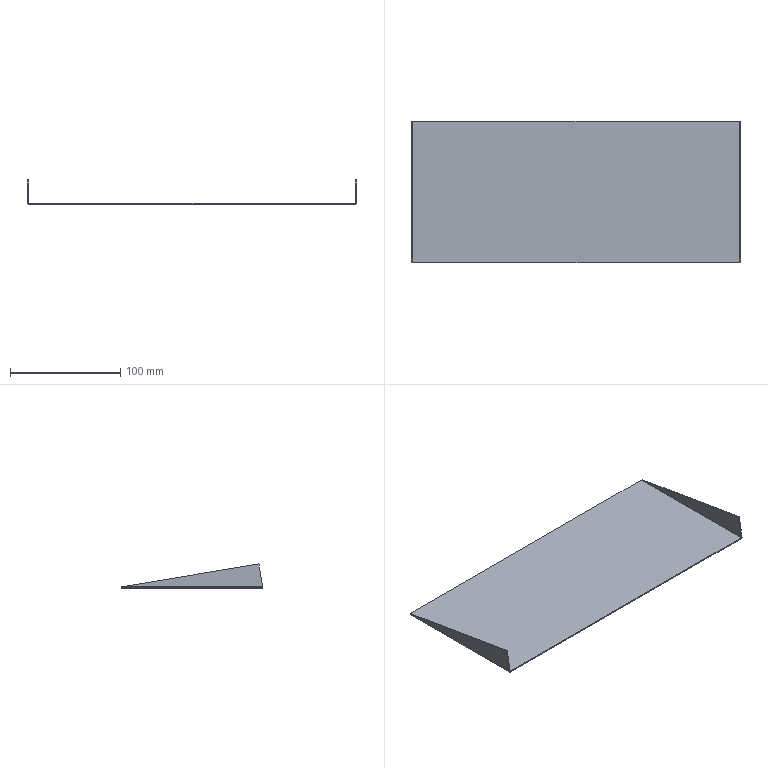Part | SolidWorks | features EdgeFlange 1, FlatPattern 1, MirrorPattern 1, SMBaseFlange 1, SheetMetal 1 | 1 solid | 20 faces | box 299 x 128.5 x 22 mm | volume 41042 mm3 | plane 12 | spline 4 | cylinder 4 | commonest cylinder face diameters 0.4 x2 2.4 x2
STEP:
#1=CARTESIAN_POINT('',(148.3,64.25,-1.));
#2=VERTEX_POINT('',#1);
#3=CARTESIAN_POINT('',(148.3,-64.25,-1.));
#4=VERTEX_POINT('',#3);
#5=CARTESIAN_POINT('',(148.3,64.25,-1.));
#6=DIRECTION('',(0.,-1.,0.));
#7=VECTOR('',#6,1000.);
#8=LINE('',#5,#7);
#9=EDGE_CURVE('',#2,#4,#8,.T.);
#10=ORIENTED_EDGE('',*,*,#9,.T.);
#11=CARTESIAN_POINT('',(-148.3,-64.25,-1.));
#12=VERTEX_POINT('',#11);
#13=CARTESIAN_POINT('',(-149.5,-64.25,-1.));
#14=DIRECTION('',(1.,0.,0.));
#15=VECTOR('',#14,1000.);
#16=LINE('',#13,#15);
#17=EDGE_CURVE('',#12,#4,#16,.T.);
#18=ORIENTED_EDGE('',*,*,#17,.F.);
#19=CARTESIAN_POINT('',(-148.3,64.25,-1.));
#20=VERTEX_POINT('',#19);
#21=CARTESIAN_POINT('',(-148.3,-64.25,-1.));
#22=DIRECTION('',(0.,1.,0.));
#23=VECTOR('',#22,1000.);
#24=LINE('',#21,#23);
#25=EDGE_CURVE('',#12,#20,#24,.T.);
#26=ORIENTED_EDGE('',*,*,#25,.T.);
#27=CARTESIAN_POINT('',(-149.5,64.25,-1.));
#28=DIRECTION('',(-1.,0.,0.));
#29=VECTOR('',#28,1000.);
#30=LINE('',#27,#29);
#31=EDGE_CURVE('',#2,#20,#30,.T.);
#32=ORIENTED_EDGE('',*,*,#31,.F.);
#33=EDGE_LOOP('',(#10,#18,#26,#32));
#34=FACE_OUTER_BOUND('',#33,.T.);
#35=CARTESIAN_POINT('',(0.,0.,-1.));
#36=DIRECTION('',(0.,0.,1.));
#37=DIRECTION('',(1.,0.,0.));
#38=AXIS2_PLACEMENT_3D('',#35,#36,#37);
#39=PLANE('',#38);
#40=ADVANCED_FACE('',(#34),#39,.F.);
#41=CARTESIAN_POINT('',(-148.3,-64.25,0.));
#42=VERTEX_POINT('',#41);
#43=CARTESIAN_POINT('',(148.3,-64.25,0.));
#44=VERTEX_POINT('',#43);
#45=CARTESIAN_POINT('',(-149.5,-64.25,0.));
#46=DIRECTION('',(1.,0.,0.));
#47=VECTOR('',#46,1000.);
#48=LINE('',#45,#47);
#49=EDGE_CURVE('',#42,#44,#48,.T.);
#50=ORIENTED_EDGE('',*,*,#49,.T.);
#51=CARTESIAN_POINT('',(148.3,64.25,0.));
#52=VERTEX_POINT('',#51);
#53=CARTESIAN_POINT('',(148.3,64.25,0.));
#54=DIRECTION('',(0.,-1.,0.));
#55=VECTOR('',#54,1000.);
#56=LINE('',#53,#55);
#57=EDGE_CURVE('',#52,#44,#56,.T.);
#58=ORIENTED_EDGE('',*,*,#57,.F.);
#59=CARTESIAN_POINT('',(-148.3,64.25,0.));
#60=VERTEX_POINT('',#59);
#61=CARTESIAN_POINT('',(-149.5,64.25,0.));
#62=DIRECTION('',(-1.,0.,0.));
#63=VECTOR('',#62,1000.);
#64=LINE('',#61,#63);
#65=EDGE_CURVE('',#52,#60,#64,.T.);
#66=ORIENTED_EDGE('',*,*,#65,.T.);
#67=CARTESIAN_POINT('',(-148.3,-64.25,0.));
#68=DIRECTION('',(0.,1.,0.));
#69=VECTOR('',#68,1000.);
#70=LINE('',#67,#69);
#71=EDGE_CURVE('',#42,#60,#70,.T.);
#72=ORIENTED_EDGE('',*,*,#71,.F.);
#73=EDGE_LOOP('',(#50,#58,#66,#72));
#74=FACE_OUTER_BOUND('',#73,.T.);
#75=CARTESIAN_POINT('',(0.,0.,0.));
#76=DIRECTION('',(0.,0.,1.));
#77=DIRECTION('',(1.,0.,0.));
#78=AXIS2_PLACEMENT_3D('',#75,#76,#77);
#79=PLANE('',#78);
#80=ADVANCED_FACE('',(#74),#79,.T.);
#81=ORIENTED_EDGE('',*,*,#65,.F.);
#82=CARTESIAN_POINT('',(148.3,64.25,0.));
#83=DIRECTION('',(0.,0.,-1.));
#84=VECTOR('',#83,1000.);
#85=LINE('',#82,#84);
#86=EDGE_CURVE('',#52,#2,#85,.T.);
#87=ORIENTED_EDGE('',*,*,#86,.T.);
#88=ORIENTED_EDGE('',*,*,#31,.T.);
#89=CARTESIAN_POINT('',(-148.3,64.25,0.));
#90=DIRECTION('',(0.,0.,-1.));
#91=VECTOR('',#90,1000.);
#92=LINE('',#89,#91);
#93=EDGE_CURVE('',#60,#20,#92,.T.);
#94=ORIENTED_EDGE('',*,*,#93,.F.);
#95=EDGE_LOOP('',(#81,#87,#88,#94));
#96=FACE_OUTER_BOUND('',#95,.T.);
#97=CARTESIAN_POINT('',(-149.5,64.25,-1.));
#98=DIRECTION('',(0.,1.,0.));
#99=DIRECTION('',(0.,0.,1.));
#100=AXIS2_PLACEMENT_3D('',#97,#98,#99);
#101=PLANE('',#100);
#102=ADVANCED_FACE('',(#96),#101,.T.);
#103=CARTESIAN_POINT('',(148.3,-64.25,0.));
#104=DIRECTION('',(0.,0.,-1.));
#105=VECTOR('',#104,1000.);
#106=LINE('',#103,#105);
#107=EDGE_CURVE('',#44,#4,#106,.T.);
#108=ORIENTED_EDGE('',*,*,#107,.F.);
#109=ORIENTED_EDGE('',*,*,#49,.F.);
#110=CARTESIAN_POINT('',(-148.3,-64.25,0.));
#111=DIRECTION('',(0.,0.,-1.));
#112=VECTOR('',#111,1000.);
#113=LINE('',#110,#112);
#114=EDGE_CURVE('',#42,#12,#113,.T.);
#115=ORIENTED_EDGE('',*,*,#114,.T.);
#116=ORIENTED_EDGE('',*,*,#17,.T.);
#117=EDGE_LOOP('',(#108,#109,#115,#116));
#118=FACE_OUTER_BOUND('',#117,.T.);
#119=CARTESIAN_POINT('',(-149.5,-64.25,-1.));
#120=DIRECTION('',(0.,-1.,0.));
#121=DIRECTION('',(0.,0.,-1.));
#122=AXIS2_PLACEMENT_3D('',#119,#120,#121);
#123=PLANE('',#122);
#124=ADVANCED_FACE('',(#118),#123,.T.);
#125=CARTESIAN_POINT('',(-148.5,63.06,0.2));
#126=VERTEX_POINT('',#125);
#127=CARTESIAN_POINT('',(-149.5,63.06,0.2));
#128=VERTEX_POINT('',#127);
#129=CARTESIAN_POINT('',(-149.5,63.06,0.2));
#130=DIRECTION('',(-1.,0.,0.));
#131=VECTOR('',#130,1000.);
#132=LINE('',#129,#131);
#133=EDGE_CURVE('',#126,#128,#132,.T.);
#134=ORIENTED_EDGE('',*,*,#133,.F.);
#135=CARTESIAN_POINT('',(-148.3,64.25,0.));
#136=CARTESIAN_POINT('',(-148.352,64.052,0.));
#137=CARTESIAN_POINT('',(-148.404,63.853,0.02155));
#138=CARTESIAN_POINT('',(-148.478,63.457,0.0956));
#139=CARTESIAN_POINT('',(-148.5,63.258,0.1476));
#140=CARTESIAN_POINT('',(-148.5,63.06,0.2));
#141=B_SPLINE_CURVE_WITH_KNOTS('',3,(#135,#136,#137,#138,#139,#140),.UNSPECIFIED.,.F.,.F.,(4,2,4),(0.,0.5,1.),.UNSPECIFIED.);
#142=EDGE_CURVE('',#60,#126,#141,.T.);
#143=ORIENTED_EDGE('',*,*,#142,.F.);
#144=ORIENTED_EDGE('',*,*,#93,.T.);
#145=CARTESIAN_POINT('',(-148.3,64.25,-1.));
#146=CARTESIAN_POINT('',(-148.459,64.15,-1.));
#147=CARTESIAN_POINT('',(-148.614,64.052,-0.9688));
#148=CARTESIAN_POINT('',(-148.906,63.852,-0.8478));
#149=CARTESIAN_POINT('',(-149.037,63.754,-0.7598));
#150=CARTESIAN_POINT('',(-149.261,63.555,-0.5362));
#151=CARTESIAN_POINT('',(-149.348,63.457,-0.4048));
#152=CARTESIAN_POINT('',(-149.469,63.257,-0.1126));
#153=CARTESIAN_POINT('',(-149.5,63.16,0.04146));
#154=CARTESIAN_POINT('',(-149.5,63.06,0.2));
#155=B_SPLINE_CURVE_WITH_KNOTS('',3,(#145,#146,#147,#148,#149,#150,#151,#152,#153,#154),.UNSPECIFIED.,.F.,.F.,(4,2,2,2,4),(0.,0.000556,0.001112,0.001668,0.002224),.UNSPECIFIED.);
#156=EDGE_CURVE('',#20,#128,#155,.T.);
#157=ORIENTED_EDGE('',*,*,#156,.T.);
#158=EDGE_LOOP('',(#134,#143,#144,#157));
#159=FACE_OUTER_BOUND('',#158,.T.);
#160=CARTESIAN_POINT('',(-148.3,64.25,-1.01));
#161=CARTESIAN_POINT('',(-148.458,64.151,-1.01));
#162=CARTESIAN_POINT('',(-148.617,64.052,-0.9785));
#163=CARTESIAN_POINT('',(-148.909,63.853,-0.8573));
#164=CARTESIAN_POINT('',(-149.044,63.754,-0.7676));
#165=CARTESIAN_POINT('',(-149.268,63.556,-0.5436));
#166=CARTESIAN_POINT('',(-149.357,63.457,-0.4094));
#167=CARTESIAN_POINT('',(-149.479,63.258,-0.1167));
#168=CARTESIAN_POINT('',(-149.51,63.159,0.04159));
#169=CARTESIAN_POINT('',(-149.51,63.06,0.2));
#170=CARTESIAN_POINT('',(-148.3,64.25,-1.));
#171=CARTESIAN_POINT('',(-148.457,64.151,-1.));
#172=CARTESIAN_POINT('',(-148.614,64.052,-0.9688));
#173=CARTESIAN_POINT('',(-148.904,63.853,-0.8485));
#174=CARTESIAN_POINT('',(-149.037,63.754,-0.7596));
#175=CARTESIAN_POINT('',(-149.26,63.556,-0.5375));
#176=CARTESIAN_POINT('',(-149.349,63.457,-0.4043));
#177=CARTESIAN_POINT('',(-149.469,63.258,-0.1141));
#178=CARTESIAN_POINT('',(-149.5,63.159,0.0429));
#179=CARTESIAN_POINT('',(-149.5,63.06,0.2));
#180=CARTESIAN_POINT('',(-148.3,64.25,0.));
#181=CARTESIAN_POINT('',(-148.326,64.151,0.));
#182=CARTESIAN_POINT('',(-148.352,64.052,0.005205));
#183=CARTESIAN_POINT('',(-148.401,63.853,0.02524));
#184=CARTESIAN_POINT('',(-148.423,63.754,0.04007));
#185=CARTESIAN_POINT('',(-148.46,63.556,0.07709));
#186=CARTESIAN_POINT('',(-148.475,63.457,0.09928));
#187=CARTESIAN_POINT('',(-148.495,63.258,0.1477));
#188=CARTESIAN_POINT('',(-148.5,63.159,0.1738));
#189=CARTESIAN_POINT('',(-148.5,63.06,0.2));
#190=B_SPLINE_SURFACE_WITH_KNOTS('',1,3,((#160,#161,#162,#163,#164,#165,#166,#167,#168,#169),(#170,#171,#172,#173,#174,#175,#176,#177,#178,#179),(#180,#181,#182,#183,#184,#185,#186,#187,#188,#189)),.UNSPECIFIED.,.F.,.F.,.F.,(2,1,2),(4,2,2,2,4),(-0.01,0.,1.),(0.,0.25,0.5,0.75,1.),.UNSPECIFIED.);
#191=ADVANCED_FACE('',(#159),#190,.F.);
#192=CARTESIAN_POINT('',(-148.5,-64.216,0.2));
#193=VERTEX_POINT('',#192);
#194=CARTESIAN_POINT('',(-148.5,-64.216,0.2));
#195=CARTESIAN_POINT('',(-148.5,-64.222,0.1476));
#196=CARTESIAN_POINT('',(-148.478,-64.228,0.0956));
#197=CARTESIAN_POINT('',(-148.404,-64.239,0.02155));
#198=CARTESIAN_POINT('',(-148.352,-64.244,0.));
#199=CARTESIAN_POINT('',(-148.3,-64.25,0.));
#200=B_SPLINE_CURVE_WITH_KNOTS('',3,(#194,#195,#196,#197,#198,#199),.UNSPECIFIED.,.F.,.F.,(4,2,4),(0.,0.5,1.),.UNSPECIFIED.);
#201=EDGE_CURVE('',#193,#42,#200,.T.);
#202=ORIENTED_EDGE('',*,*,#201,.F.);
#203=CARTESIAN_POINT('',(-149.5,-64.216,0.2));
#204=VERTEX_POINT('',#203);
#205=CARTESIAN_POINT('',(-148.5,-64.216,0.2));
#206=DIRECTION('',(-1.,0.,0.));
#207=VECTOR('',#206,1000.);
#208=LINE('',#205,#207);
#209=EDGE_CURVE('',#193,#204,#208,.T.);
#210=ORIENTED_EDGE('',*,*,#209,.T.);
#211=CARTESIAN_POINT('',(-149.5,-64.216,0.2));
#212=CARTESIAN_POINT('',(-149.5,-64.219,0.04292));
#213=CARTESIAN_POINT('',(-149.469,-64.222,-0.1141));
#214=CARTESIAN_POINT('',(-149.349,-64.228,-0.4043));
#215=CARTESIAN_POINT('',(-149.26,-64.23,-0.5375));
#216=CARTESIAN_POINT('',(-149.037,-64.236,-0.7596));
#217=CARTESIAN_POINT('',(-148.904,-64.239,-0.8485));
#218=CARTESIAN_POINT('',(-148.614,-64.244,-0.9688));
#219=CARTESIAN_POINT('',(-148.457,-64.247,-1.));
#220=CARTESIAN_POINT('',(-148.3,-64.25,-1.));
#221=B_SPLINE_CURVE_WITH_KNOTS('',3,(#211,#212,#213,#214,#215,#216,#217,#218,#219,#220),.UNSPECIFIED.,.F.,.F.,(4,2,2,2,4),(0.,0.25,0.5,0.75,1.),.UNSPECIFIED.);
#222=EDGE_CURVE('',#204,#12,#221,.T.);
#223=ORIENTED_EDGE('',*,*,#222,.T.);
#224=ORIENTED_EDGE('',*,*,#114,.F.);
#225=EDGE_LOOP('',(#202,#210,#223,#224));
#226=FACE_OUTER_BOUND('',#225,.T.);
#227=CARTESIAN_POINT('',(-149.51,-64.216,0.2));
#228=CARTESIAN_POINT('',(-149.51,-64.219,0.04158));
#229=CARTESIAN_POINT('',(-149.479,-64.222,-0.1167));
#230=CARTESIAN_POINT('',(-149.357,-64.228,-0.4094));
#231=CARTESIAN_POINT('',(-149.268,-64.23,-0.5436));
#232=CARTESIAN_POINT('',(-149.044,-64.236,-0.7676));
#233=CARTESIAN_POINT('',(-148.909,-64.239,-0.8573));
#234=CARTESIAN_POINT('',(-148.617,-64.244,-0.9785));
#235=CARTESIAN_POINT('',(-148.458,-64.247,-1.01));
#236=CARTESIAN_POINT('',(-148.3,-64.25,-1.01));
#237=CARTESIAN_POINT('',(-149.5,-64.216,0.2));
#238=CARTESIAN_POINT('',(-149.5,-64.219,0.04289));
#239=CARTESIAN_POINT('',(-149.469,-64.222,-0.1141));
#240=CARTESIAN_POINT('',(-149.349,-64.228,-0.4043));
#241=CARTESIAN_POINT('',(-149.26,-64.23,-0.5375));
#242=CARTESIAN_POINT('',(-149.037,-64.236,-0.7596));
#243=CARTESIAN_POINT('',(-148.904,-64.239,-0.8485));
#244=CARTESIAN_POINT('',(-148.614,-64.244,-0.9688));
#245=CARTESIAN_POINT('',(-148.457,-64.247,-1.));
#246=CARTESIAN_POINT('',(-148.3,-64.25,-1.));
#247=CARTESIAN_POINT('',(-148.5,-64.216,0.2));
#248=CARTESIAN_POINT('',(-148.5,-64.219,0.1738));
#249=CARTESIAN_POINT('',(-148.495,-64.222,0.1477));
#250=CARTESIAN_POINT('',(-148.475,-64.228,0.09928));
#251=CARTESIAN_POINT('',(-148.46,-64.23,0.07709));
#252=CARTESIAN_POINT('',(-148.423,-64.236,0.04007));
#253=CARTESIAN_POINT('',(-148.401,-64.239,0.02524));
#254=CARTESIAN_POINT('',(-148.352,-64.244,0.005205));
#255=CARTESIAN_POINT('',(-148.326,-64.247,0.));
#256=CARTESIAN_POINT('',(-148.3,-64.25,0.));
#257=CARTESIAN_POINT('',(-148.49,-64.216,0.2));
#258=CARTESIAN_POINT('',(-148.49,-64.219,0.1751));
#259=CARTESIAN_POINT('',(-148.485,-64.222,0.1503));
#260=CARTESIAN_POINT('',(-148.466,-64.228,0.1044));
#261=CARTESIAN_POINT('',(-148.452,-64.23,0.0833));
#262=CARTESIAN_POINT('',(-148.417,-64.236,0.04814));
#263=CARTESIAN_POINT('',(-148.396,-64.239,0.03407));
#264=CARTESIAN_POINT('',(-148.35,-64.244,0.01504));
#265=CARTESIAN_POINT('',(-148.325,-64.247,0.0101));
#266=CARTESIAN_POINT('',(-148.3,-64.25,0.0101));
#267=B_SPLINE_SURFACE_WITH_KNOTS('',1,3,((#227,#228,#229,#230,#231,#232,#233,#234,#235,#236),(#237,#238,#239,#240,#241,#242,#243,#244,#245,#246),(#247,#248,#249,#250,#251,#252,#253,#254,#255,#256),(#257,#258,#259,#260,#261,#262,#263,#264,#265,#266)),.UNSPECIFIED.,.F.,.F.,.F.,(2,1,1,2),(4,2,2,2,4),(-0.01,0.,1.,1.01),(0.,0.25,0.5,0.75,1.),.UNSPECIFIED.);
#268=ADVANCED_FACE('',(#226),#267,.F.);
#269=ORIENTED_EDGE('',*,*,#25,.F.);
#270=ORIENTED_EDGE('',*,*,#222,.F.);
#271=CARTESIAN_POINT('',(-149.5,63.06,0.2));
#272=DIRECTION('',(0.,1.,0.));
#273=VECTOR('',#272,1000.);
#274=LINE('',#271,#273);
#275=EDGE_CURVE('',#204,#128,#274,.T.);
#276=ORIENTED_EDGE('',*,*,#275,.T.);
#277=ORIENTED_EDGE('',*,*,#156,.F.);
#278=EDGE_LOOP('',(#269,#270,#276,#277));
#279=FACE_OUTER_BOUND('',#278,.T.);
#280=CARTESIAN_POINT('',(-148.3,-64.25,0.2));
#281=DIRECTION('',(0.,-1.,0.));
#282=DIRECTION('',(-1.,0.,0.));
#283=AXIS2_PLACEMENT_3D('',#280,#281,#282);
#284=CYLINDRICAL_SURFACE('',#283,1.2);
#285=ADVANCED_FACE('',(#279),#284,.T.);
#286=ORIENTED_EDGE('',*,*,#71,.T.);
#287=ORIENTED_EDGE('',*,*,#142,.T.);
#288=CARTESIAN_POINT('',(-148.5,63.06,0.2));
#289=DIRECTION('',(0.,-1.,0.));
#290=VECTOR('',#289,1000.);
#291=LINE('',#288,#290);
#292=EDGE_CURVE('',#126,#193,#291,.T.);
#293=ORIENTED_EDGE('',*,*,#292,.T.);
#294=ORIENTED_EDGE('',*,*,#201,.T.);
#295=EDGE_LOOP('',(#286,#287,#293,#294));
#296=FACE_OUTER_BOUND('',#295,.T.);
#297=CARTESIAN_POINT('',(-148.3,-64.25,0.2));
#298=DIRECTION('',(0.,-1.,0.));
#299=DIRECTION('',(-1.,0.,0.));
#300=AXIS2_PLACEMENT_3D('',#297,#298,#299);
#301=CYLINDRICAL_SURFACE('',#300,0.2);
#302=ADVANCED_FACE('',(#296),#301,.F.);
#303=ORIENTED_EDGE('',*,*,#133,.T.);
#304=CARTESIAN_POINT('',(-149.5,-60.721,21.));
#305=VERTEX_POINT('',#304);
#306=CARTESIAN_POINT('',(-149.5,1.764,10.5));
#307=DIRECTION('',(0.,0.9862,-0.1657));
#308=VECTOR('',#307,1000.);
#309=LINE('',#306,#308);
#310=EDGE_CURVE('',#305,#128,#309,.T.);
#311=ORIENTED_EDGE('',*,*,#310,.F.);
#312=CARTESIAN_POINT('',(-148.5,-60.721,21.));
#313=VERTEX_POINT('',#312);
#314=CARTESIAN_POINT('',(-149.5,-60.721,21.));
#315=DIRECTION('',(1.,0.,0.));
#316=VECTOR('',#315,1000.);
#317=LINE('',#314,#316);
#318=EDGE_CURVE('',#305,#313,#317,.T.);
#319=ORIENTED_EDGE('',*,*,#318,.T.);
#320=CARTESIAN_POINT('',(-148.5,-60.721,21.));
#321=DIRECTION('',(0.,0.9862,-0.1657));
#322=VECTOR('',#321,1000.);
#323=LINE('',#320,#322);
#324=EDGE_CURVE('',#313,#126,#323,.T.);
#325=ORIENTED_EDGE('',*,*,#324,.T.);
#326=EDGE_LOOP('',(#303,#311,#319,#325));
#327=FACE_OUTER_BOUND('',#326,.T.);
#328=CARTESIAN_POINT('',(-149.5,-60.721,21.));
#329=DIRECTION('',(0.,-0.1657,-0.9862));
#330=DIRECTION('',(0.,0.9862,-0.1657));
#331=AXIS2_PLACEMENT_3D('',#328,#329,#330);
#332=PLANE('',#331);
#333=ADVANCED_FACE('',(#327),#332,.F.);
#334=ORIENTED_EDGE('',*,*,#209,.F.);
#335=CARTESIAN_POINT('',(-148.5,-64.25,0.));
#336=DIRECTION('',(0.,0.1657,0.9862));
#337=VECTOR('',#336,1000.);
#338=LINE('',#335,#337);
#339=EDGE_CURVE('',#193,#313,#338,.T.);
#340=ORIENTED_EDGE('',*,*,#339,.T.);
#341=ORIENTED_EDGE('',*,*,#318,.F.);
#342=CARTESIAN_POINT('',(-149.5,-62.486,10.5));
#343=DIRECTION('',(0.,0.1657,0.9862));
#344=VECTOR('',#343,1000.);
#345=LINE('',#342,#344);
#346=EDGE_CURVE('',#204,#305,#345,.T.);
#347=ORIENTED_EDGE('',*,*,#346,.F.);
#348=EDGE_LOOP('',(#334,#340,#341,#347));
#349=FACE_OUTER_BOUND('',#348,.T.);
#350=CARTESIAN_POINT('',(-149.5,-64.25,0.));
#351=DIRECTION('',(0.,0.9862,-0.1657));
#352=DIRECTION('',(0.,0.1657,0.9862));
#353=AXIS2_PLACEMENT_3D('',#350,#351,#352);
#354=PLANE('',#353);
#355=ADVANCED_FACE('',(#349),#354,.F.);
#356=ORIENTED_EDGE('',*,*,#275,.F.);
#357=ORIENTED_EDGE('',*,*,#346,.T.);
#358=ORIENTED_EDGE('',*,*,#310,.T.);
#359=EDGE_LOOP('',(#356,#357,#358));
#360=FACE_OUTER_BOUND('',#359,.T.);
#361=CARTESIAN_POINT('',(-149.5,0.,0.));
#362=DIRECTION('',(1.,0.,0.));
#363=DIRECTION('',(0.,0.,-1.));
#364=AXIS2_PLACEMENT_3D('',#361,#362,#363);
#365=PLANE('',#364);
#366=ADVANCED_FACE('',(#360),#365,.F.);
#367=ORIENTED_EDGE('',*,*,#339,.F.);
#368=ORIENTED_EDGE('',*,*,#292,.F.);
#369=ORIENTED_EDGE('',*,*,#324,.F.);
#370=EDGE_LOOP('',(#367,#368,#369));
#371=FACE_OUTER_BOUND('',#370,.T.);
#372=CARTESIAN_POINT('',(-148.5,0.,0.));
#373=DIRECTION('',(1.,0.,0.));
#374=DIRECTION('',(0.,0.,-1.));
#375=AXIS2_PLACEMENT_3D('',#372,#373,#374);
#376=PLANE('',#375);
#377=ADVANCED_FACE('',(#371),#376,.T.);
#378=CARTESIAN_POINT('',(148.5,-64.216,0.2));
#379=VERTEX_POINT('',#378);
#380=CARTESIAN_POINT('',(149.5,-64.216,0.2));
#381=VERTEX_POINT('',#380);
#382=CARTESIAN_POINT('',(149.5,-64.216,0.2));
#383=DIRECTION('',(1.,0.,0.));
#384=VECTOR('',#383,1000.);
#385=LINE('',#382,#384);
#386=EDGE_CURVE('',#379,#381,#385,.T.);
#387=ORIENTED_EDGE('',*,*,#386,.F.);
#388=CARTESIAN_POINT('',(148.3,-64.25,0.));
#389=CARTESIAN_POINT('',(148.352,-64.244,0.));
#390=CARTESIAN_POINT('',(148.404,-64.239,0.02155));
#391=CARTESIAN_POINT('',(148.478,-64.228,0.0956));
#392=CARTESIAN_POINT('',(148.5,-64.222,0.1476));
#393=CARTESIAN_POINT('',(148.5,-64.216,0.2));
#394=B_SPLINE_CURVE_WITH_KNOTS('',3,(#388,#389,#390,#391,#392,#393),.UNSPECIFIED.,.F.,.F.,(4,2,4),(0.,0.5,1.),.UNSPECIFIED.);
#395=EDGE_CURVE('',#44,#379,#394,.T.);
#396=ORIENTED_EDGE('',*,*,#395,.F.);
#397=ORIENTED_EDGE('',*,*,#107,.T.);
#398=CARTESIAN_POINT('',(148.3,-64.25,-1.));
#399=CARTESIAN_POINT('',(148.457,-64.247,-1.));
#400=CARTESIAN_POINT('',(148.614,-64.244,-0.9688));
#401=CARTESIAN_POINT('',(148.904,-64.239,-0.8485));
#402=CARTESIAN_POINT('',(149.037,-64.236,-0.7596));
#403=CARTESIAN_POINT('',(149.26,-64.23,-0.5375));
#404=CARTESIAN_POINT('',(149.349,-64.228,-0.4043));
#405=CARTESIAN_POINT('',(149.469,-64.222,-0.1141));
#406=CARTESIAN_POINT('',(149.5,-64.219,0.04292));
#407=CARTESIAN_POINT('',(149.5,-64.216,0.2));
#408=B_SPLINE_CURVE_WITH_KNOTS('',3,(#398,#399,#400,#401,#402,#403,#404,#405,#406,#407),.UNSPECIFIED.,.F.,.F.,(4,2,2,2,4),(0.,0.25,0.5,0.75,1.),.UNSPECIFIED.);
#409=EDGE_CURVE('',#4,#381,#408,.T.);
#410=ORIENTED_EDGE('',*,*,#409,.T.);
#411=EDGE_LOOP('',(#387,#396,#397,#410));
#412=FACE_OUTER_BOUND('',#411,.T.);
#413=CARTESIAN_POINT('',(148.3,-64.25,-1.01));
#414=CARTESIAN_POINT('',(148.458,-64.247,-1.01));
#415=CARTESIAN_POINT('',(148.617,-64.244,-0.9785));
#416=CARTESIAN_POINT('',(148.909,-64.239,-0.8573));
#417=CARTESIAN_POINT('',(149.044,-64.236,-0.7676));
#418=CARTESIAN_POINT('',(149.268,-64.23,-0.5436));
#419=CARTESIAN_POINT('',(149.357,-64.228,-0.4094));
#420=CARTESIAN_POINT('',(149.479,-64.222,-0.1167));
#421=CARTESIAN_POINT('',(149.51,-64.219,0.04158));
#422=CARTESIAN_POINT('',(149.51,-64.216,0.2));
#423=CARTESIAN_POINT('',(148.3,-64.25,-1.));
#424=CARTESIAN_POINT('',(148.457,-64.247,-1.));
#425=CARTESIAN_POINT('',(148.614,-64.244,-0.9688));
#426=CARTESIAN_POINT('',(148.904,-64.239,-0.8485));
#427=CARTESIAN_POINT('',(149.037,-64.236,-0.7596));
#428=CARTESIAN_POINT('',(149.26,-64.23,-0.5375));
#429=CARTESIAN_POINT('',(149.349,-64.228,-0.4043));
#430=CARTESIAN_POINT('',(149.469,-64.222,-0.1141));
#431=CARTESIAN_POINT('',(149.5,-64.219,0.04289));
#432=CARTESIAN_POINT('',(149.5,-64.216,0.2));
#433=CARTESIAN_POINT('',(148.3,-64.25,0.));
#434=CARTESIAN_POINT('',(148.326,-64.247,0.));
#435=CARTESIAN_POINT('',(148.352,-64.244,0.005205));
#436=CARTESIAN_POINT('',(148.401,-64.239,0.02524));
#437=CARTESIAN_POINT('',(148.423,-64.236,0.04007));
#438=CARTESIAN_POINT('',(148.46,-64.23,0.07709));
#439=CARTESIAN_POINT('',(148.475,-64.228,0.09928));
#440=CARTESIAN_POINT('',(148.495,-64.222,0.1477));
#441=CARTESIAN_POINT('',(148.5,-64.219,0.1738));
#442=CARTESIAN_POINT('',(148.5,-64.216,0.2));
#443=CARTESIAN_POINT('',(148.3,-64.25,0.0101));
#444=CARTESIAN_POINT('',(148.325,-64.247,0.0101));
#445=CARTESIAN_POINT('',(148.35,-64.244,0.01504));
#446=CARTESIAN_POINT('',(148.396,-64.239,0.03407));
#447=CARTESIAN_POINT('',(148.417,-64.236,0.04814));
#448=CARTESIAN_POINT('',(148.452,-64.23,0.0833));
#449=CARTESIAN_POINT('',(148.466,-64.228,0.1044));
#450=CARTESIAN_POINT('',(148.485,-64.222,0.1503));
#451=CARTESIAN_POINT('',(148.49,-64.219,0.1751));
#452=CARTESIAN_POINT('',(148.49,-64.216,0.2));
#453=B_SPLINE_SURFACE_WITH_KNOTS('',1,3,((#413,#414,#415,#416,#417,#418,#419,#420,#421,#422),(#423,#424,#425,#426,#427,#428,#429,#430,#431,#432),(#433,#434,#435,#436,#437,#438,#439,#440,#441,#442),(#443,#444,#445,#446,#447,#448,#449,#450,#451,#452)),.UNSPECIFIED.,.F.,.F.,.F.,(2,1,1,2),(4,2,2,2,4),(-0.01,0.,1.,1.01),(0.,0.25,0.5,0.75,1.),.UNSPECIFIED.);
#454=ADVANCED_FACE('',(#412),#453,.F.);
#455=CARTESIAN_POINT('',(148.5,63.06,0.2));
#456=VERTEX_POINT('',#455);
#457=CARTESIAN_POINT('',(148.5,63.06,0.2));
#458=CARTESIAN_POINT('',(148.5,63.258,0.1476));
#459=CARTESIAN_POINT('',(148.478,63.457,0.0956));
#460=CARTESIAN_POINT('',(148.404,63.853,0.02155));
#461=CARTESIAN_POINT('',(148.352,64.052,0.));
#462=CARTESIAN_POINT('',(148.3,64.25,0.));
#463=B_SPLINE_CURVE_WITH_KNOTS('',3,(#457,#458,#459,#460,#461,#462),.UNSPECIFIED.,.F.,.F.,(4,2,4),(0.,0.5,1.),.UNSPECIFIED.);
#464=EDGE_CURVE('',#456,#52,#463,.T.);
#465=ORIENTED_EDGE('',*,*,#464,.F.);
#466=CARTESIAN_POINT('',(149.5,63.06,0.2));
#467=VERTEX_POINT('',#466);
#468=CARTESIAN_POINT('',(148.5,63.06,0.2));
#469=DIRECTION('',(1.,0.,0.));
#470=VECTOR('',#469,1000.);
#471=LINE('',#468,#470);
#472=EDGE_CURVE('',#456,#467,#471,.T.);
#473=ORIENTED_EDGE('',*,*,#472,.T.);
#474=CARTESIAN_POINT('',(149.5,63.06,0.2));
#475=CARTESIAN_POINT('',(149.5,63.16,0.04146));
#476=CARTESIAN_POINT('',(149.469,63.258,-0.1143));
#477=CARTESIAN_POINT('',(149.348,63.458,-0.4059));
#478=CARTESIAN_POINT('',(149.26,63.556,-0.5374));
#479=CARTESIAN_POINT('',(149.036,63.755,-0.7607));
#480=CARTESIAN_POINT('',(148.905,63.853,-0.8484));
#481=CARTESIAN_POINT('',(148.613,64.053,-0.9693));
#482=CARTESIAN_POINT('',(148.459,64.15,-1.));
#483=CARTESIAN_POINT('',(148.3,64.25,-1.));
#484=B_SPLINE_CURVE_WITH_KNOTS('',3,(#474,#475,#476,#477,#478,#479,#480,#481,#482,#483),.UNSPECIFIED.,.F.,.F.,(4,2,2,2,4),(0.,0.000556,0.001112,0.001668,0.002224),.UNSPECIFIED.);
#485=EDGE_CURVE('',#467,#2,#484,.T.);
#486=ORIENTED_EDGE('',*,*,#485,.T.);
#487=ORIENTED_EDGE('',*,*,#86,.F.);
#488=EDGE_LOOP('',(#465,#473,#486,#487));
#489=FACE_OUTER_BOUND('',#488,.T.);
#490=CARTESIAN_POINT('',(149.51,63.06,0.2));
#491=CARTESIAN_POINT('',(149.51,63.159,0.04159));
#492=CARTESIAN_POINT('',(149.479,63.258,-0.1167));
#493=CARTESIAN_POINT('',(149.357,63.457,-0.4094));
#494=CARTESIAN_POINT('',(149.268,63.556,-0.5436));
#495=CARTESIAN_POINT('',(149.044,63.754,-0.7676));
#496=CARTESIAN_POINT('',(148.909,63.853,-0.8573));
#497=CARTESIAN_POINT('',(148.617,64.052,-0.9785));
#498=CARTESIAN_POINT('',(148.458,64.151,-1.01));
#499=CARTESIAN_POINT('',(148.3,64.25,-1.01));
#500=CARTESIAN_POINT('',(149.5,63.06,0.2));
#501=CARTESIAN_POINT('',(149.5,63.159,0.0429));
#502=CARTESIAN_POINT('',(149.469,63.258,-0.1141));
#503=CARTESIAN_POINT('',(149.349,63.457,-0.4043));
#504=CARTESIAN_POINT('',(149.26,63.556,-0.5375));
#505=CARTESIAN_POINT('',(149.037,63.754,-0.7596));
#506=CARTESIAN_POINT('',(148.904,63.853,-0.8485));
#507=CARTESIAN_POINT('',(148.614,64.052,-0.9688));
#508=CARTESIAN_POINT('',(148.457,64.151,-1.));
#509=CARTESIAN_POINT('',(148.3,64.25,-1.));
#510=CARTESIAN_POINT('',(148.5,63.06,0.2));
#511=CARTESIAN_POINT('',(148.5,63.159,0.1738));
#512=CARTESIAN_POINT('',(148.495,63.258,0.1477));
#513=CARTESIAN_POINT('',(148.475,63.457,0.09928));
#514=CARTESIAN_POINT('',(148.46,63.556,0.07709));
#515=CARTESIAN_POINT('',(148.423,63.754,0.04007));
#516=CARTESIAN_POINT('',(148.401,63.853,0.02524));
#517=CARTESIAN_POINT('',(148.352,64.052,0.005205));
#518=CARTESIAN_POINT('',(148.326,64.151,0.));
#519=CARTESIAN_POINT('',(148.3,64.25,0.));
#520=B_SPLINE_SURFACE_WITH_KNOTS('',1,3,((#490,#491,#492,#493,#494,#495,#496,#497,#498,#499),(#500,#501,#502,#503,#504,#505,#506,#507,#508,#509),(#510,#511,#512,#513,#514,#515,#516,#517,#518,#519)),.UNSPECIFIED.,.F.,.F.,.F.,(2,1,2),(4,2,2,2,4),(-0.01,0.,1.),(0.,0.25,0.5,0.75,1.),.UNSPECIFIED.);
#521=ADVANCED_FACE('',(#489),#520,.F.);
#522=ORIENTED_EDGE('',*,*,#9,.F.);
#523=ORIENTED_EDGE('',*,*,#485,.F.);
#524=CARTESIAN_POINT('',(149.5,-64.216,0.2));
#525=DIRECTION('',(0.,-1.,0.));
#526=VECTOR('',#525,1000.);
#527=LINE('',#524,#526);
#528=EDGE_CURVE('',#467,#381,#527,.T.);
#529=ORIENTED_EDGE('',*,*,#528,.T.);
#530=ORIENTED_EDGE('',*,*,#409,.F.);
#531=EDGE_LOOP('',(#522,#523,#529,#530));
#532=FACE_OUTER_BOUND('',#531,.T.);
#533=CARTESIAN_POINT('',(148.3,64.25,0.2));
#534=DIRECTION('',(0.,1.,0.));
#535=DIRECTION('',(1.,0.,0.));
#536=AXIS2_PLACEMENT_3D('',#533,#534,#535);
#537=CYLINDRICAL_SURFACE('',#536,1.2);
#538=ADVANCED_FACE('',(#532),#537,.T.);
#539=ORIENTED_EDGE('',*,*,#57,.T.);
#540=ORIENTED_EDGE('',*,*,#395,.T.);
#541=CARTESIAN_POINT('',(148.5,-64.216,0.2));
#542=DIRECTION('',(0.,1.,0.));
#543=VECTOR('',#542,1000.);
#544=LINE('',#541,#543);
#545=EDGE_CURVE('',#379,#456,#544,.T.);
#546=ORIENTED_EDGE('',*,*,#545,.T.);
#547=ORIENTED_EDGE('',*,*,#464,.T.);
#548=EDGE_LOOP('',(#539,#540,#546,#547));
#549=FACE_OUTER_BOUND('',#548,.T.);
#550=CARTESIAN_POINT('',(148.3,64.25,0.2));
#551=DIRECTION('',(0.,1.,0.));
#552=DIRECTION('',(1.,0.,0.));
#553=AXIS2_PLACEMENT_3D('',#550,#551,#552);
#554=CYLINDRICAL_SURFACE('',#553,0.2);
#555=ADVANCED_FACE('',(#549),#554,.F.);
#556=CARTESIAN_POINT('',(149.5,-60.721,21.));
#557=VERTEX_POINT('',#556);
#558=CARTESIAN_POINT('',(149.5,-60.721,21.));
#559=DIRECTION('',(0.,0.9862,-0.1657));
#560=VECTOR('',#559,1000.);
#561=LINE('',#558,#560);
#562=EDGE_CURVE('',#557,#467,#561,.T.);
#563=ORIENTED_EDGE('',*,*,#562,.T.);
#564=ORIENTED_EDGE('',*,*,#472,.F.);
#565=CARTESIAN_POINT('',(148.5,-60.721,21.));
#566=VERTEX_POINT('',#565);
#567=CARTESIAN_POINT('',(148.5,1.764,10.5));
#568=DIRECTION('',(0.,0.9862,-0.1657));
#569=VECTOR('',#568,1000.);
#570=LINE('',#567,#569);
#571=EDGE_CURVE('',#566,#456,#570,.T.);
#572=ORIENTED_EDGE('',*,*,#571,.F.);
#573=CARTESIAN_POINT('',(149.5,-60.721,21.));
#574=DIRECTION('',(-1.,0.,0.));
#575=VECTOR('',#574,1000.);
#576=LINE('',#573,#575);
#577=EDGE_CURVE('',#557,#566,#576,.T.);
#578=ORIENTED_EDGE('',*,*,#577,.F.);
#579=EDGE_LOOP('',(#563,#564,#572,#578));
#580=FACE_OUTER_BOUND('',#579,.T.);
#581=CARTESIAN_POINT('',(149.5,-60.721,21.));
#582=DIRECTION('',(0.,0.1657,0.9862));
#583=DIRECTION('',(0.,-0.9862,0.1657));
#584=AXIS2_PLACEMENT_3D('',#581,#582,#583);
#585=PLANE('',#584);
#586=ADVANCED_FACE('',(#580),#585,.T.);
#587=CARTESIAN_POINT('',(148.5,-62.486,10.5));
#588=DIRECTION('',(0.,0.1657,0.9862));
#589=VECTOR('',#588,1000.);
#590=LINE('',#587,#589);
#591=EDGE_CURVE('',#379,#566,#590,.T.);
#592=ORIENTED_EDGE('',*,*,#591,.F.);
#593=ORIENTED_EDGE('',*,*,#386,.T.);
#594=CARTESIAN_POINT('',(149.5,-64.25,0.));
#595=DIRECTION('',(0.,0.1657,0.9862));
#596=VECTOR('',#595,1000.);
#597=LINE('',#594,#596);
#598=EDGE_CURVE('',#381,#557,#597,.T.);
#599=ORIENTED_EDGE('',*,*,#598,.T.);
#600=ORIENTED_EDGE('',*,*,#577,.T.);
#601=EDGE_LOOP('',(#592,#593,#599,#600));
#602=FACE_OUTER_BOUND('',#601,.T.);
#603=CARTESIAN_POINT('',(149.5,-64.25,0.));
#604=DIRECTION('',(0.,-0.9862,0.1657));
#605=DIRECTION('',(0.,-0.1657,-0.9862));
#606=AXIS2_PLACEMENT_3D('',#603,#604,#605);
#607=PLANE('',#606);
#608=ADVANCED_FACE('',(#602),#607,.T.);
#609=ORIENTED_EDGE('',*,*,#528,.F.);
#610=ORIENTED_EDGE('',*,*,#562,.F.);
#611=ORIENTED_EDGE('',*,*,#598,.F.);
#612=EDGE_LOOP('',(#609,#610,#611));
#613=FACE_OUTER_BOUND('',#612,.T.);
#614=CARTESIAN_POINT('',(149.5,0.,0.));
#615=DIRECTION('',(-1.,0.,0.));
#616=DIRECTION('',(0.,0.,-1.));
#617=AXIS2_PLACEMENT_3D('',#614,#615,#616);
#618=PLANE('',#617);
#619=ADVANCED_FACE('',(#613),#618,.F.);
#620=ORIENTED_EDGE('',*,*,#571,.T.);
#621=ORIENTED_EDGE('',*,*,#545,.F.);
#622=ORIENTED_EDGE('',*,*,#591,.T.);
#623=EDGE_LOOP('',(#620,#621,#622));
#624=FACE_OUTER_BOUND('',#623,.T.);
#625=CARTESIAN_POINT('',(148.5,0.,0.));
#626=DIRECTION('',(-1.,0.,0.));
#627=DIRECTION('',(0.,0.,-1.));
#628=AXIS2_PLACEMENT_3D('',#625,#626,#627);
#629=PLANE('',#628);
#630=ADVANCED_FACE('',(#624),#629,.T.);
#631=CLOSED_SHELL('',(#40,#80,#102,#124,#191,#268,#285,#302,#333,#355,#366,#377,#454,#521,#538,#555,#586,#608,#619,#630));
#632=MANIFOLD_SOLID_BREP('',#631);
#633=CARTESIAN_POINT('',(0.,0.,0.));
#634=DIRECTION('',(0.,0.,1.));
#635=DIRECTION('',(1.,0.,0.));
#636=AXIS2_PLACEMENT_3D('',#633,#634,#635);
#637=(LENGTH_UNIT()NAMED_UNIT(*)SI_UNIT(.MILLI.,.METRE.));
#638=UNCERTAINTY_MEASURE_WITH_UNIT(LENGTH_MEASURE(0.00001),#637,'','');
#639=(NAMED_UNIT(*)PLANE_ANGLE_UNIT()SI_UNIT($,.RADIAN.));
#640=(NAMED_UNIT(*)SI_UNIT($,.STERADIAN.)SOLID_ANGLE_UNIT());
#641=(GEOMETRIC_REPRESENTATION_CONTEXT(3)GLOBAL_UNCERTAINTY_ASSIGNED_CONTEXT((#638))GLOBAL_UNIT_ASSIGNED_CONTEXT((#637,#639,#640))REPRESENTATION_CONTEXT('',''));
#642=ADVANCED_BREP_SHAPE_REPRESENTATION('',(#632,#636),#641);